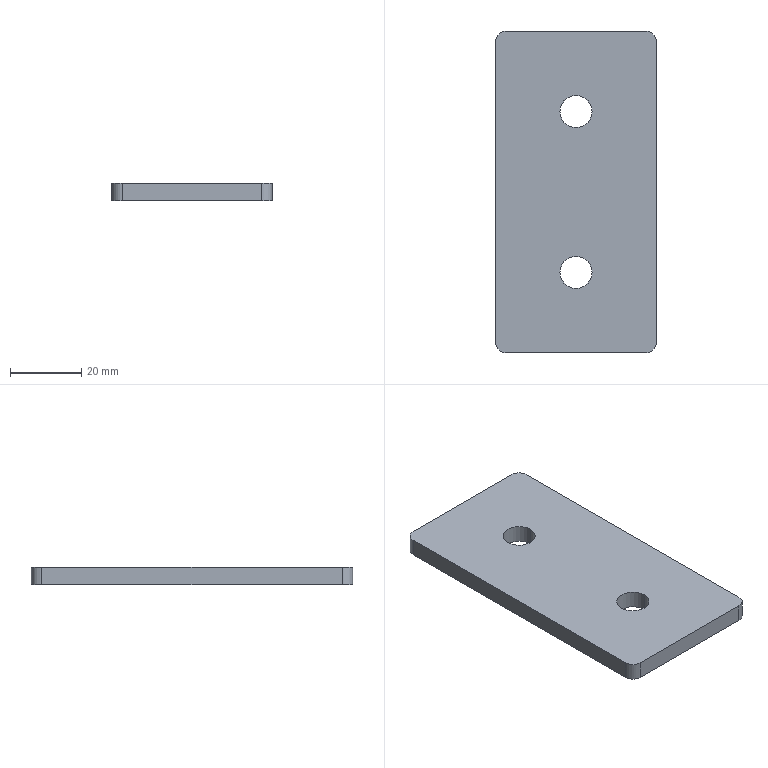Part | STEP file | 1 solid | 14 faces | box 45 x 90 x 5 mm | volume 19575 mm3 | cylinder 8 | plane 6 | commonest cylinder face diameters 6 x4 9 x4
STEP:
#1=CARTESIAN_POINT('',(0.,0.,0.));
#2=DIRECTION('',(0.,0.,1.));
#3=DIRECTION('',(1.,0.,0.));
#4=AXIS2_PLACEMENT_3D('',#1,#2,#3);
#5=CARTESIAN_POINT('',(-545.5,-331.5,5.));
#6=VERTEX_POINT('',#5);
#7=CARTESIAN_POINT('',(-554.5,-331.5,5.));
#8=VERTEX_POINT('',#7);
#9=CARTESIAN_POINT('',(-550.,-331.5,5.));
#10=DIRECTION('',(0.,0.,1.));
#11=DIRECTION('',(1.,0.,0.));
#12=AXIS2_PLACEMENT_3D('',#9,#10,#11);
#13=CIRCLE('',#12,4.5);
#14=CARTESIAN_POINT('',(-550.,-331.5,0.));
#15=DIRECTION('',(0.,0.,1.));
#16=DIRECTION('',(1.,0.,0.));
#17=AXIS2_PLACEMENT_3D('',#14,#15,#16);
#18=CYLINDRICAL_SURFACE('',#17,4.5);
#19=CARTESIAN_POINT('',(0.,5.));
#20=DIRECTION('',(1.,0.));
#21=VECTOR('',#20,1.);
#22=LINE('',#19,#21);
#23=(GEOMETRIC_REPRESENTATION_CONTEXT(2)PARAMETRIC_REPRESENTATION_CONTEXT()REPRESENTATION_CONTEXT('',''));
#24=DEFINITIONAL_REPRESENTATION('',(#22),#23);
#25=PCURVE('',#18,#24);
#26=CARTESIAN_POINT('',(-569.5,-267.,5.));
#27=DIRECTION('',(0.,0.,1.));
#28=DIRECTION('',(1.,0.,0.));
#29=AXIS2_PLACEMENT_3D('',#26,#27,#28);
#30=PLANE('',#29);
#31=CARTESIAN_POINT('',(19.5,-64.5));
#32=DIRECTION('',(1.,0.));
#33=AXIS2_PLACEMENT_2D('',#31,#32);
#34=CIRCLE('',#33,4.5);
#35=(GEOMETRIC_REPRESENTATION_CONTEXT(2)PARAMETRIC_REPRESENTATION_CONTEXT()REPRESENTATION_CONTEXT('',''));
#36=DEFINITIONAL_REPRESENTATION('',(#34),#35);
#37=PCURVE('',#30,#36);
#38=SURFACE_CURVE('',#13,(#25,#37),.PCURVE_S1.);
#39=EDGE_CURVE('',#6,#8,#38,.T.);
#40=ORIENTED_EDGE('',*,*,#39,.F.);
#41=CARTESIAN_POINT('',(-545.5,-331.5,0.));
#42=VERTEX_POINT('',#41);
#43=CARTESIAN_POINT('',(-545.5,-331.5,0.));
#44=DIRECTION('',(0.,0.,1.));
#45=VECTOR('',#44,1.);
#46=LINE('',#43,#45);
#47=CARTESIAN_POINT('',(0.,0.));
#48=DIRECTION('',(0.,1.));
#49=VECTOR('',#48,1.);
#50=LINE('',#47,#49);
#51=(GEOMETRIC_REPRESENTATION_CONTEXT(2)PARAMETRIC_REPRESENTATION_CONTEXT()REPRESENTATION_CONTEXT('',''));
#52=DEFINITIONAL_REPRESENTATION('',(#50),#51);
#53=PCURVE('',#18,#52);
#54=CARTESIAN_POINT('',(-550.,-331.5,0.));
#55=DIRECTION('',(0.,0.,1.));
#56=DIRECTION('',(1.,0.,0.));
#57=AXIS2_PLACEMENT_3D('',#54,#55,#56);
#58=CYLINDRICAL_SURFACE('',#57,4.5);
#59=CARTESIAN_POINT('',(6.283,0.));
#60=DIRECTION('',(0.,1.));
#61=VECTOR('',#60,1.);
#62=LINE('',#59,#61);
#63=(GEOMETRIC_REPRESENTATION_CONTEXT(2)PARAMETRIC_REPRESENTATION_CONTEXT()REPRESENTATION_CONTEXT('',''));
#64=DEFINITIONAL_REPRESENTATION('',(#62),#63);
#65=PCURVE('',#58,#64);
#66=SURFACE_CURVE('',#46,(#53,#65),.PCURVE_S1.);
#67=EDGE_CURVE('',#42,#6,#66,.T.);
#68=ORIENTED_EDGE('',*,*,#67,.F.);
#69=CARTESIAN_POINT('',(-554.5,-331.5,0.));
#70=VERTEX_POINT('',#69);
#71=CARTESIAN_POINT('',(-550.,-331.5,0.));
#72=DIRECTION('',(0.,0.,1.));
#73=DIRECTION('',(1.,0.,0.));
#74=AXIS2_PLACEMENT_3D('',#71,#72,#73);
#75=CIRCLE('',#74,4.5);
#76=CARTESIAN_POINT('',(0.,0.));
#77=DIRECTION('',(1.,0.));
#78=VECTOR('',#77,1.);
#79=LINE('',#76,#78);
#80=(GEOMETRIC_REPRESENTATION_CONTEXT(2)PARAMETRIC_REPRESENTATION_CONTEXT()REPRESENTATION_CONTEXT('',''));
#81=DEFINITIONAL_REPRESENTATION('',(#79),#80);
#82=PCURVE('',#18,#81);
#83=CARTESIAN_POINT('',(-569.5,-267.,0.));
#84=DIRECTION('',(0.,0.,1.));
#85=DIRECTION('',(1.,0.,0.));
#86=AXIS2_PLACEMENT_3D('',#83,#84,#85);
#87=PLANE('',#86);
#88=CARTESIAN_POINT('',(19.5,-64.5));
#89=DIRECTION('',(1.,0.));
#90=AXIS2_PLACEMENT_2D('',#88,#89);
#91=CIRCLE('',#90,4.5);
#92=(GEOMETRIC_REPRESENTATION_CONTEXT(2)PARAMETRIC_REPRESENTATION_CONTEXT()REPRESENTATION_CONTEXT('',''));
#93=DEFINITIONAL_REPRESENTATION('',(#91),#92);
#94=PCURVE('',#87,#93);
#95=SURFACE_CURVE('',#75,(#82,#94),.PCURVE_S1.);
#96=EDGE_CURVE('',#42,#70,#95,.T.);
#97=ORIENTED_EDGE('',*,*,#96,.T.);
#98=CARTESIAN_POINT('',(-554.5,-331.5,0.));
#99=DIRECTION('',(0.,0.,1.));
#100=VECTOR('',#99,1.);
#101=LINE('',#98,#100);
#102=CARTESIAN_POINT('',(3.142,0.));
#103=DIRECTION('',(0.,1.));
#104=VECTOR('',#103,1.);
#105=LINE('',#102,#104);
#106=(GEOMETRIC_REPRESENTATION_CONTEXT(2)PARAMETRIC_REPRESENTATION_CONTEXT()REPRESENTATION_CONTEXT('',''));
#107=DEFINITIONAL_REPRESENTATION('',(#105),#106);
#108=PCURVE('',#18,#107);
#109=CARTESIAN_POINT('',(3.142,0.));
#110=DIRECTION('',(0.,1.));
#111=VECTOR('',#110,1.);
#112=LINE('',#109,#111);
#113=(GEOMETRIC_REPRESENTATION_CONTEXT(2)PARAMETRIC_REPRESENTATION_CONTEXT()REPRESENTATION_CONTEXT('',''));
#114=DEFINITIONAL_REPRESENTATION('',(#112),#113);
#115=PCURVE('',#58,#114);
#116=SURFACE_CURVE('',#101,(#108,#115),.PCURVE_S1.);
#117=EDGE_CURVE('',#70,#8,#116,.T.);
#118=ORIENTED_EDGE('',*,*,#117,.T.);
#119=EDGE_LOOP('',(#40,#68,#97,#118));
#120=FACE_BOUND('',#119,.F.);
#121=ADVANCED_FACE('',(#120),#18,.F.);
#122=CARTESIAN_POINT('',(-545.5,-286.5,5.));
#123=VERTEX_POINT('',#122);
#124=CARTESIAN_POINT('',(-554.5,-286.5,5.));
#125=VERTEX_POINT('',#124);
#126=CARTESIAN_POINT('',(-550.,-286.5,5.));
#127=DIRECTION('',(0.,0.,1.));
#128=DIRECTION('',(1.,0.,0.));
#129=AXIS2_PLACEMENT_3D('',#126,#127,#128);
#130=CIRCLE('',#129,4.5);
#131=CARTESIAN_POINT('',(-550.,-286.5,0.));
#132=DIRECTION('',(0.,0.,1.));
#133=DIRECTION('',(1.,0.,0.));
#134=AXIS2_PLACEMENT_3D('',#131,#132,#133);
#135=CYLINDRICAL_SURFACE('',#134,4.5);
#136=CARTESIAN_POINT('',(0.,5.));
#137=DIRECTION('',(1.,0.));
#138=VECTOR('',#137,1.);
#139=LINE('',#136,#138);
#140=(GEOMETRIC_REPRESENTATION_CONTEXT(2)PARAMETRIC_REPRESENTATION_CONTEXT()REPRESENTATION_CONTEXT('',''));
#141=DEFINITIONAL_REPRESENTATION('',(#139),#140);
#142=PCURVE('',#135,#141);
#143=CARTESIAN_POINT('',(19.5,-19.5));
#144=DIRECTION('',(1.,0.));
#145=AXIS2_PLACEMENT_2D('',#143,#144);
#146=CIRCLE('',#145,4.5);
#147=(GEOMETRIC_REPRESENTATION_CONTEXT(2)PARAMETRIC_REPRESENTATION_CONTEXT()REPRESENTATION_CONTEXT('',''));
#148=DEFINITIONAL_REPRESENTATION('',(#146),#147);
#149=PCURVE('',#30,#148);
#150=SURFACE_CURVE('',#130,(#142,#149),.PCURVE_S1.);
#151=EDGE_CURVE('',#123,#125,#150,.T.);
#152=ORIENTED_EDGE('',*,*,#151,.F.);
#153=CARTESIAN_POINT('',(-545.5,-286.5,0.));
#154=VERTEX_POINT('',#153);
#155=CARTESIAN_POINT('',(-545.5,-286.5,0.));
#156=DIRECTION('',(0.,0.,1.));
#157=VECTOR('',#156,1.);
#158=LINE('',#155,#157);
#159=CARTESIAN_POINT('',(0.,0.));
#160=DIRECTION('',(0.,1.));
#161=VECTOR('',#160,1.);
#162=LINE('',#159,#161);
#163=(GEOMETRIC_REPRESENTATION_CONTEXT(2)PARAMETRIC_REPRESENTATION_CONTEXT()REPRESENTATION_CONTEXT('',''));
#164=DEFINITIONAL_REPRESENTATION('',(#162),#163);
#165=PCURVE('',#135,#164);
#166=CARTESIAN_POINT('',(-550.,-286.5,0.));
#167=DIRECTION('',(0.,0.,1.));
#168=DIRECTION('',(1.,0.,0.));
#169=AXIS2_PLACEMENT_3D('',#166,#167,#168);
#170=CYLINDRICAL_SURFACE('',#169,4.5);
#171=CARTESIAN_POINT('',(6.283,0.));
#172=DIRECTION('',(0.,1.));
#173=VECTOR('',#172,1.);
#174=LINE('',#171,#173);
#175=(GEOMETRIC_REPRESENTATION_CONTEXT(2)PARAMETRIC_REPRESENTATION_CONTEXT()REPRESENTATION_CONTEXT('',''));
#176=DEFINITIONAL_REPRESENTATION('',(#174),#175);
#177=PCURVE('',#170,#176);
#178=SURFACE_CURVE('',#158,(#165,#177),.PCURVE_S1.);
#179=EDGE_CURVE('',#154,#123,#178,.T.);
#180=ORIENTED_EDGE('',*,*,#179,.F.);
#181=CARTESIAN_POINT('',(-554.5,-286.5,0.));
#182=VERTEX_POINT('',#181);
#183=CARTESIAN_POINT('',(-550.,-286.5,0.));
#184=DIRECTION('',(0.,0.,1.));
#185=DIRECTION('',(1.,0.,0.));
#186=AXIS2_PLACEMENT_3D('',#183,#184,#185);
#187=CIRCLE('',#186,4.5);
#188=CARTESIAN_POINT('',(0.,0.));
#189=DIRECTION('',(1.,0.));
#190=VECTOR('',#189,1.);
#191=LINE('',#188,#190);
#192=(GEOMETRIC_REPRESENTATION_CONTEXT(2)PARAMETRIC_REPRESENTATION_CONTEXT()REPRESENTATION_CONTEXT('',''));
#193=DEFINITIONAL_REPRESENTATION('',(#191),#192);
#194=PCURVE('',#135,#193);
#195=CARTESIAN_POINT('',(19.5,-19.5));
#196=DIRECTION('',(1.,0.));
#197=AXIS2_PLACEMENT_2D('',#195,#196);
#198=CIRCLE('',#197,4.5);
#199=(GEOMETRIC_REPRESENTATION_CONTEXT(2)PARAMETRIC_REPRESENTATION_CONTEXT()REPRESENTATION_CONTEXT('',''));
#200=DEFINITIONAL_REPRESENTATION('',(#198),#199);
#201=PCURVE('',#87,#200);
#202=SURFACE_CURVE('',#187,(#194,#201),.PCURVE_S1.);
#203=EDGE_CURVE('',#154,#182,#202,.T.);
#204=ORIENTED_EDGE('',*,*,#203,.T.);
#205=CARTESIAN_POINT('',(-554.5,-286.5,0.));
#206=DIRECTION('',(0.,0.,1.));
#207=VECTOR('',#206,1.);
#208=LINE('',#205,#207);
#209=CARTESIAN_POINT('',(3.142,0.));
#210=DIRECTION('',(0.,1.));
#211=VECTOR('',#210,1.);
#212=LINE('',#209,#211);
#213=(GEOMETRIC_REPRESENTATION_CONTEXT(2)PARAMETRIC_REPRESENTATION_CONTEXT()REPRESENTATION_CONTEXT('',''));
#214=DEFINITIONAL_REPRESENTATION('',(#212),#213);
#215=PCURVE('',#135,#214);
#216=CARTESIAN_POINT('',(3.142,0.));
#217=DIRECTION('',(0.,1.));
#218=VECTOR('',#217,1.);
#219=LINE('',#216,#218);
#220=(GEOMETRIC_REPRESENTATION_CONTEXT(2)PARAMETRIC_REPRESENTATION_CONTEXT()REPRESENTATION_CONTEXT('',''));
#221=DEFINITIONAL_REPRESENTATION('',(#219),#220);
#222=PCURVE('',#170,#221);
#223=SURFACE_CURVE('',#208,(#215,#222),.PCURVE_S1.);
#224=EDGE_CURVE('',#182,#125,#223,.T.);
#225=ORIENTED_EDGE('',*,*,#224,.T.);
#226=EDGE_LOOP('',(#152,#180,#204,#225));
#227=FACE_BOUND('',#226,.F.);
#228=ADVANCED_FACE('',(#227),#135,.F.);
#229=ORIENTED_EDGE('',*,*,#203,.T.);
#230=CARTESIAN_POINT('',(-550.,-286.5,0.));
#231=DIRECTION('',(0.,0.,1.));
#232=DIRECTION('',(1.,0.,0.));
#233=AXIS2_PLACEMENT_3D('',#230,#231,#232);
#234=CIRCLE('',#233,4.5);
#235=CARTESIAN_POINT('',(19.5,-19.5));
#236=DIRECTION('',(1.,0.));
#237=AXIS2_PLACEMENT_2D('',#235,#236);
#238=CIRCLE('',#237,4.5);
#239=(GEOMETRIC_REPRESENTATION_CONTEXT(2)PARAMETRIC_REPRESENTATION_CONTEXT()REPRESENTATION_CONTEXT('',''));
#240=DEFINITIONAL_REPRESENTATION('',(#238),#239);
#241=PCURVE('',#87,#240);
#242=CARTESIAN_POINT('',(0.,0.));
#243=DIRECTION('',(1.,0.));
#244=VECTOR('',#243,1.);
#245=LINE('',#242,#244);
#246=(GEOMETRIC_REPRESENTATION_CONTEXT(2)PARAMETRIC_REPRESENTATION_CONTEXT()REPRESENTATION_CONTEXT('',''));
#247=DEFINITIONAL_REPRESENTATION('',(#245),#246);
#248=PCURVE('',#170,#247);
#249=SURFACE_CURVE('',#234,(#241,#248),.PCURVE_S1.);
#250=EDGE_CURVE('',#182,#154,#249,.T.);
#251=ORIENTED_EDGE('',*,*,#250,.T.);
#252=EDGE_LOOP('',(#229,#251));
#253=FACE_BOUND('',#252,.T.);
#254=ORIENTED_EDGE('',*,*,#96,.T.);
#255=CARTESIAN_POINT('',(-550.,-331.5,0.));
#256=DIRECTION('',(0.,0.,1.));
#257=DIRECTION('',(1.,0.,0.));
#258=AXIS2_PLACEMENT_3D('',#255,#256,#257);
#259=CIRCLE('',#258,4.5);
#260=CARTESIAN_POINT('',(19.5,-64.5));
#261=DIRECTION('',(1.,0.));
#262=AXIS2_PLACEMENT_2D('',#260,#261);
#263=CIRCLE('',#262,4.5);
#264=(GEOMETRIC_REPRESENTATION_CONTEXT(2)PARAMETRIC_REPRESENTATION_CONTEXT()REPRESENTATION_CONTEXT('',''));
#265=DEFINITIONAL_REPRESENTATION('',(#263),#264);
#266=PCURVE('',#87,#265);
#267=CARTESIAN_POINT('',(0.,0.));
#268=DIRECTION('',(1.,0.));
#269=VECTOR('',#268,1.);
#270=LINE('',#267,#269);
#271=(GEOMETRIC_REPRESENTATION_CONTEXT(2)PARAMETRIC_REPRESENTATION_CONTEXT()REPRESENTATION_CONTEXT('',''));
#272=DEFINITIONAL_REPRESENTATION('',(#270),#271);
#273=PCURVE('',#58,#272);
#274=SURFACE_CURVE('',#259,(#266,#273),.PCURVE_S1.);
#275=EDGE_CURVE('',#70,#42,#274,.T.);
#276=ORIENTED_EDGE('',*,*,#275,.T.);
#277=EDGE_LOOP('',(#254,#276));
#278=FACE_BOUND('',#277,.T.);
#279=CARTESIAN_POINT('',(-569.5,-264.,0.));
#280=VERTEX_POINT('',#279);
#281=CARTESIAN_POINT('',(-572.5,-267.,0.));
#282=VERTEX_POINT('',#281);
#283=CARTESIAN_POINT('',(-569.5,-267.,0.));
#284=DIRECTION('',(0.,0.,1.));
#285=DIRECTION('',(1.,0.,0.));
#286=AXIS2_PLACEMENT_3D('',#283,#284,#285);
#287=CIRCLE('',#286,3.);
#288=CARTESIAN_POINT('',(0.,0.));
#289=DIRECTION('',(1.,0.));
#290=AXIS2_PLACEMENT_2D('',#288,#289);
#291=CIRCLE('',#290,3.);
#292=(GEOMETRIC_REPRESENTATION_CONTEXT(2)PARAMETRIC_REPRESENTATION_CONTEXT()REPRESENTATION_CONTEXT('',''));
#293=DEFINITIONAL_REPRESENTATION('',(#291),#292);
#294=PCURVE('',#87,#293);
#295=CARTESIAN_POINT('',(-569.5,-267.,5.));
#296=DIRECTION('',(0.,0.,-1.));
#297=DIRECTION('',(-1.,0.,0.));
#298=AXIS2_PLACEMENT_3D('',#295,#296,#297);
#299=CYLINDRICAL_SURFACE('',#298,3.);
#300=CARTESIAN_POINT('',(3.142,5.));
#301=DIRECTION('',(-1.,0.));
#302=VECTOR('',#301,1.);
#303=LINE('',#300,#302);
#304=(GEOMETRIC_REPRESENTATION_CONTEXT(2)PARAMETRIC_REPRESENTATION_CONTEXT()REPRESENTATION_CONTEXT('',''));
#305=DEFINITIONAL_REPRESENTATION('',(#303),#304);
#306=PCURVE('',#299,#305);
#307=SURFACE_CURVE('',#287,(#294,#306),.PCURVE_S1.);
#308=EDGE_CURVE('',#280,#282,#307,.T.);
#309=ORIENTED_EDGE('',*,*,#308,.F.);
#310=CARTESIAN_POINT('',(-530.5,-264.,0.));
#311=VERTEX_POINT('',#310);
#312=CARTESIAN_POINT('',(-530.5,-264.,0.));
#313=DIRECTION('',(-1.,0.,0.));
#314=VECTOR('',#313,1.);
#315=LINE('',#312,#314);
#316=CARTESIAN_POINT('',(39.,3.));
#317=DIRECTION('',(-1.,0.));
#318=VECTOR('',#317,1.);
#319=LINE('',#316,#318);
#320=(GEOMETRIC_REPRESENTATION_CONTEXT(2)PARAMETRIC_REPRESENTATION_CONTEXT()REPRESENTATION_CONTEXT('',''));
#321=DEFINITIONAL_REPRESENTATION('',(#319),#320);
#322=PCURVE('',#87,#321);
#323=CARTESIAN_POINT('',(-530.5,-264.,5.));
#324=DIRECTION('',(0.,-1.,0.));
#325=DIRECTION('',(0.,0.,-1.));
#326=AXIS2_PLACEMENT_3D('',#323,#324,#325);
#327=PLANE('',#326);
#328=CARTESIAN_POINT('',(5.,0.));
#329=DIRECTION('',(0.,-1.));
#330=VECTOR('',#329,1.);
#331=LINE('',#328,#330);
#332=(GEOMETRIC_REPRESENTATION_CONTEXT(2)PARAMETRIC_REPRESENTATION_CONTEXT()REPRESENTATION_CONTEXT('',''));
#333=DEFINITIONAL_REPRESENTATION('',(#331),#332);
#334=PCURVE('',#327,#333);
#335=SURFACE_CURVE('',#315,(#322,#334),.PCURVE_S1.);
#336=EDGE_CURVE('',#311,#280,#335,.T.);
#337=ORIENTED_EDGE('',*,*,#336,.F.);
#338=CARTESIAN_POINT('',(-527.5,-267.,0.));
#339=VERTEX_POINT('',#338);
#340=CARTESIAN_POINT('',(-530.5,-267.,0.));
#341=DIRECTION('',(0.,0.,1.));
#342=DIRECTION('',(-1.,0.,0.));
#343=AXIS2_PLACEMENT_3D('',#340,#341,#342);
#344=CIRCLE('',#343,3.);
#345=CARTESIAN_POINT('',(39.,0.));
#346=DIRECTION('',(-1.,0.));
#347=AXIS2_PLACEMENT_2D('',#345,#346);
#348=CIRCLE('',#347,3.);
#349=(GEOMETRIC_REPRESENTATION_CONTEXT(2)PARAMETRIC_REPRESENTATION_CONTEXT()REPRESENTATION_CONTEXT('',''));
#350=DEFINITIONAL_REPRESENTATION('',(#348),#349);
#351=PCURVE('',#87,#350);
#352=CARTESIAN_POINT('',(-530.5,-267.,5.));
#353=DIRECTION('',(0.,0.,-1.));
#354=DIRECTION('',(-1.,0.,0.));
#355=AXIS2_PLACEMENT_3D('',#352,#353,#354);
#356=CYLINDRICAL_SURFACE('',#355,3.);
#357=CARTESIAN_POINT('',(6.283,5.));
#358=DIRECTION('',(-1.,0.));
#359=VECTOR('',#358,1.);
#360=LINE('',#357,#359);
#361=(GEOMETRIC_REPRESENTATION_CONTEXT(2)PARAMETRIC_REPRESENTATION_CONTEXT()REPRESENTATION_CONTEXT('',''));
#362=DEFINITIONAL_REPRESENTATION('',(#360),#361);
#363=PCURVE('',#356,#362);
#364=SURFACE_CURVE('',#344,(#351,#363),.PCURVE_S1.);
#365=EDGE_CURVE('',#339,#311,#364,.T.);
#366=ORIENTED_EDGE('',*,*,#365,.F.);
#367=CARTESIAN_POINT('',(-527.5,-351.,0.));
#368=VERTEX_POINT('',#367);
#369=CARTESIAN_POINT('',(-527.5,-267.,0.));
#370=DIRECTION('',(0.,1.,0.));
#371=VECTOR('',#370,1.);
#372=LINE('',#369,#371);
#373=CARTESIAN_POINT('',(42.,0.));
#374=DIRECTION('',(0.,1.));
#375=VECTOR('',#374,1.);
#376=LINE('',#373,#375);
#377=(GEOMETRIC_REPRESENTATION_CONTEXT(2)PARAMETRIC_REPRESENTATION_CONTEXT()REPRESENTATION_CONTEXT('',''));
#378=DEFINITIONAL_REPRESENTATION('',(#376),#377);
#379=PCURVE('',#87,#378);
#380=CARTESIAN_POINT('',(-527.5,-267.,5.));
#381=DIRECTION('',(-1.,0.,0.));
#382=DIRECTION('',(0.,0.,1.));
#383=AXIS2_PLACEMENT_3D('',#380,#381,#382);
#384=PLANE('',#383);
#385=CARTESIAN_POINT('',(-5.,0.));
#386=DIRECTION('',(0.,1.));
#387=VECTOR('',#386,1.);
#388=LINE('',#385,#387);
#389=(GEOMETRIC_REPRESENTATION_CONTEXT(2)PARAMETRIC_REPRESENTATION_CONTEXT()REPRESENTATION_CONTEXT('',''));
#390=DEFINITIONAL_REPRESENTATION('',(#388),#389);
#391=PCURVE('',#384,#390);
#392=SURFACE_CURVE('',#372,(#379,#391),.PCURVE_S1.);
#393=EDGE_CURVE('',#368,#339,#392,.T.);
#394=ORIENTED_EDGE('',*,*,#393,.F.);
#395=CARTESIAN_POINT('',(-530.5,-354.,0.));
#396=VERTEX_POINT('',#395);
#397=CARTESIAN_POINT('',(-530.5,-351.,0.));
#398=DIRECTION('',(0.,0.,1.));
#399=DIRECTION('',(-1.,0.,0.));
#400=AXIS2_PLACEMENT_3D('',#397,#398,#399);
#401=CIRCLE('',#400,3.);
#402=CARTESIAN_POINT('',(39.,-84.));
#403=DIRECTION('',(-1.,0.));
#404=AXIS2_PLACEMENT_2D('',#402,#403);
#405=CIRCLE('',#404,3.);
#406=(GEOMETRIC_REPRESENTATION_CONTEXT(2)PARAMETRIC_REPRESENTATION_CONTEXT()REPRESENTATION_CONTEXT('',''));
#407=DEFINITIONAL_REPRESENTATION('',(#405),#406);
#408=PCURVE('',#87,#407);
#409=CARTESIAN_POINT('',(-530.5,-351.,5.));
#410=DIRECTION('',(0.,0.,-1.));
#411=DIRECTION('',(-1.,0.,0.));
#412=AXIS2_PLACEMENT_3D('',#409,#410,#411);
#413=CYLINDRICAL_SURFACE('',#412,3.);
#414=CARTESIAN_POINT('',(6.283,5.));
#415=DIRECTION('',(-1.,0.));
#416=VECTOR('',#415,1.);
#417=LINE('',#414,#416);
#418=(GEOMETRIC_REPRESENTATION_CONTEXT(2)PARAMETRIC_REPRESENTATION_CONTEXT()REPRESENTATION_CONTEXT('',''));
#419=DEFINITIONAL_REPRESENTATION('',(#417),#418);
#420=PCURVE('',#413,#419);
#421=SURFACE_CURVE('',#401,(#408,#420),.PCURVE_S1.);
#422=EDGE_CURVE('',#396,#368,#421,.T.);
#423=ORIENTED_EDGE('',*,*,#422,.F.);
#424=CARTESIAN_POINT('',(-569.5,-354.,0.));
#425=VERTEX_POINT('',#424);
#426=CARTESIAN_POINT('',(-530.5,-354.,0.));
#427=DIRECTION('',(1.,0.,0.));
#428=VECTOR('',#427,1.);
#429=LINE('',#426,#428);
#430=CARTESIAN_POINT('',(39.,-87.));
#431=DIRECTION('',(1.,0.));
#432=VECTOR('',#431,1.);
#433=LINE('',#430,#432);
#434=(GEOMETRIC_REPRESENTATION_CONTEXT(2)PARAMETRIC_REPRESENTATION_CONTEXT()REPRESENTATION_CONTEXT('',''));
#435=DEFINITIONAL_REPRESENTATION('',(#433),#434);
#436=PCURVE('',#87,#435);
#437=CARTESIAN_POINT('',(-530.5,-354.,5.));
#438=DIRECTION('',(0.,1.,0.));
#439=DIRECTION('',(1.,0.,0.));
#440=AXIS2_PLACEMENT_3D('',#437,#438,#439);
#441=PLANE('',#440);
#442=CARTESIAN_POINT('',(0.,5.));
#443=DIRECTION('',(1.,0.));
#444=VECTOR('',#443,1.);
#445=LINE('',#442,#444);
#446=(GEOMETRIC_REPRESENTATION_CONTEXT(2)PARAMETRIC_REPRESENTATION_CONTEXT()REPRESENTATION_CONTEXT('',''));
#447=DEFINITIONAL_REPRESENTATION('',(#445),#446);
#448=PCURVE('',#441,#447);
#449=SURFACE_CURVE('',#429,(#436,#448),.PCURVE_S1.);
#450=EDGE_CURVE('',#425,#396,#449,.T.);
#451=ORIENTED_EDGE('',*,*,#450,.F.);
#452=CARTESIAN_POINT('',(-572.5,-351.,0.));
#453=VERTEX_POINT('',#452);
#454=CARTESIAN_POINT('',(-569.5,-351.,0.));
#455=DIRECTION('',(0.,0.,1.));
#456=DIRECTION('',(-1.,0.,0.));
#457=AXIS2_PLACEMENT_3D('',#454,#455,#456);
#458=CIRCLE('',#457,3.);
#459=CARTESIAN_POINT('',(0.,-84.));
#460=DIRECTION('',(-1.,0.));
#461=AXIS2_PLACEMENT_2D('',#459,#460);
#462=CIRCLE('',#461,3.);
#463=(GEOMETRIC_REPRESENTATION_CONTEXT(2)PARAMETRIC_REPRESENTATION_CONTEXT()REPRESENTATION_CONTEXT('',''));
#464=DEFINITIONAL_REPRESENTATION('',(#462),#463);
#465=PCURVE('',#87,#464);
#466=CARTESIAN_POINT('',(-569.5,-351.,5.));
#467=DIRECTION('',(0.,0.,-1.));
#468=DIRECTION('',(-1.,0.,0.));
#469=AXIS2_PLACEMENT_3D('',#466,#467,#468);
#470=CYLINDRICAL_SURFACE('',#469,3.);
#471=CARTESIAN_POINT('',(6.283,5.));
#472=DIRECTION('',(-1.,0.));
#473=VECTOR('',#472,1.);
#474=LINE('',#471,#473);
#475=(GEOMETRIC_REPRESENTATION_CONTEXT(2)PARAMETRIC_REPRESENTATION_CONTEXT()REPRESENTATION_CONTEXT('',''));
#476=DEFINITIONAL_REPRESENTATION('',(#474),#475);
#477=PCURVE('',#470,#476);
#478=SURFACE_CURVE('',#458,(#465,#477),.PCURVE_S1.);
#479=EDGE_CURVE('',#453,#425,#478,.T.);
#480=ORIENTED_EDGE('',*,*,#479,.F.);
#481=CARTESIAN_POINT('',(-572.5,-267.,0.));
#482=DIRECTION('',(0.,-1.,0.));
#483=VECTOR('',#482,1.);
#484=LINE('',#481,#483);
#485=CARTESIAN_POINT('',(-3.,0.));
#486=DIRECTION('',(0.,-1.));
#487=VECTOR('',#486,1.);
#488=LINE('',#485,#487);
#489=(GEOMETRIC_REPRESENTATION_CONTEXT(2)PARAMETRIC_REPRESENTATION_CONTEXT()REPRESENTATION_CONTEXT('',''));
#490=DEFINITIONAL_REPRESENTATION('',(#488),#489);
#491=PCURVE('',#87,#490);
#492=CARTESIAN_POINT('',(-572.5,-267.,5.));
#493=DIRECTION('',(1.,0.,0.));
#494=DIRECTION('',(0.,1.,0.));
#495=AXIS2_PLACEMENT_3D('',#492,#493,#494);
#496=PLANE('',#495);
#497=CARTESIAN_POINT('',(0.,-5.));
#498=DIRECTION('',(-1.,0.));
#499=VECTOR('',#498,1.);
#500=LINE('',#497,#499);
#501=(GEOMETRIC_REPRESENTATION_CONTEXT(2)PARAMETRIC_REPRESENTATION_CONTEXT()REPRESENTATION_CONTEXT('',''));
#502=DEFINITIONAL_REPRESENTATION('',(#500),#501);
#503=PCURVE('',#496,#502);
#504=SURFACE_CURVE('',#484,(#491,#503),.PCURVE_S1.);
#505=EDGE_CURVE('',#282,#453,#504,.T.);
#506=ORIENTED_EDGE('',*,*,#505,.F.);
#507=EDGE_LOOP('',(#309,#337,#366,#394,#423,#451,#480,#506));
#508=FACE_BOUND('',#507,.T.);
#509=ADVANCED_FACE('',(#253,#278,#508),#87,.F.);
#510=ORIENTED_EDGE('',*,*,#151,.F.);
#511=CARTESIAN_POINT('',(-550.,-286.5,5.));
#512=DIRECTION('',(0.,0.,1.));
#513=DIRECTION('',(1.,0.,0.));
#514=AXIS2_PLACEMENT_3D('',#511,#512,#513);
#515=CIRCLE('',#514,4.5);
#516=CARTESIAN_POINT('',(19.5,-19.5));
#517=DIRECTION('',(1.,0.));
#518=AXIS2_PLACEMENT_2D('',#516,#517);
#519=CIRCLE('',#518,4.5);
#520=(GEOMETRIC_REPRESENTATION_CONTEXT(2)PARAMETRIC_REPRESENTATION_CONTEXT()REPRESENTATION_CONTEXT('',''));
#521=DEFINITIONAL_REPRESENTATION('',(#519),#520);
#522=PCURVE('',#30,#521);
#523=CARTESIAN_POINT('',(0.,5.));
#524=DIRECTION('',(1.,0.));
#525=VECTOR('',#524,1.);
#526=LINE('',#523,#525);
#527=(GEOMETRIC_REPRESENTATION_CONTEXT(2)PARAMETRIC_REPRESENTATION_CONTEXT()REPRESENTATION_CONTEXT('',''));
#528=DEFINITIONAL_REPRESENTATION('',(#526),#527);
#529=PCURVE('',#170,#528);
#530=SURFACE_CURVE('',#515,(#522,#529),.PCURVE_S1.);
#531=EDGE_CURVE('',#125,#123,#530,.T.);
#532=ORIENTED_EDGE('',*,*,#531,.F.);
#533=EDGE_LOOP('',(#510,#532));
#534=FACE_BOUND('',#533,.T.);
#535=ORIENTED_EDGE('',*,*,#39,.F.);
#536=CARTESIAN_POINT('',(-550.,-331.5,5.));
#537=DIRECTION('',(0.,0.,1.));
#538=DIRECTION('',(1.,0.,0.));
#539=AXIS2_PLACEMENT_3D('',#536,#537,#538);
#540=CIRCLE('',#539,4.5);
#541=CARTESIAN_POINT('',(19.5,-64.5));
#542=DIRECTION('',(1.,0.));
#543=AXIS2_PLACEMENT_2D('',#541,#542);
#544=CIRCLE('',#543,4.5);
#545=(GEOMETRIC_REPRESENTATION_CONTEXT(2)PARAMETRIC_REPRESENTATION_CONTEXT()REPRESENTATION_CONTEXT('',''));
#546=DEFINITIONAL_REPRESENTATION('',(#544),#545);
#547=PCURVE('',#30,#546);
#548=CARTESIAN_POINT('',(0.,5.));
#549=DIRECTION('',(1.,0.));
#550=VECTOR('',#549,1.);
#551=LINE('',#548,#550);
#552=(GEOMETRIC_REPRESENTATION_CONTEXT(2)PARAMETRIC_REPRESENTATION_CONTEXT()REPRESENTATION_CONTEXT('',''));
#553=DEFINITIONAL_REPRESENTATION('',(#551),#552);
#554=PCURVE('',#58,#553);
#555=SURFACE_CURVE('',#540,(#547,#554),.PCURVE_S1.);
#556=EDGE_CURVE('',#8,#6,#555,.T.);
#557=ORIENTED_EDGE('',*,*,#556,.F.);
#558=EDGE_LOOP('',(#535,#557));
#559=FACE_BOUND('',#558,.T.);
#560=CARTESIAN_POINT('',(-569.5,-264.,5.));
#561=VERTEX_POINT('',#560);
#562=CARTESIAN_POINT('',(-572.5,-267.,5.));
#563=VERTEX_POINT('',#562);
#564=CARTESIAN_POINT('',(-569.5,-267.,5.));
#565=DIRECTION('',(0.,0.,1.));
#566=DIRECTION('',(1.,0.,0.));
#567=AXIS2_PLACEMENT_3D('',#564,#565,#566);
#568=CIRCLE('',#567,3.);
#569=CARTESIAN_POINT('',(0.,0.));
#570=DIRECTION('',(1.,0.));
#571=AXIS2_PLACEMENT_2D('',#569,#570);
#572=CIRCLE('',#571,3.);
#573=(GEOMETRIC_REPRESENTATION_CONTEXT(2)PARAMETRIC_REPRESENTATION_CONTEXT()REPRESENTATION_CONTEXT('',''));
#574=DEFINITIONAL_REPRESENTATION('',(#572),#573);
#575=PCURVE('',#30,#574);
#576=CARTESIAN_POINT('',(3.142,0.));
#577=DIRECTION('',(-1.,0.));
#578=VECTOR('',#577,1.);
#579=LINE('',#576,#578);
#580=(GEOMETRIC_REPRESENTATION_CONTEXT(2)PARAMETRIC_REPRESENTATION_CONTEXT()REPRESENTATION_CONTEXT('',''));
#581=DEFINITIONAL_REPRESENTATION('',(#579),#580);
#582=PCURVE('',#299,#581);
#583=SURFACE_CURVE('',#568,(#575,#582),.PCURVE_S1.);
#584=EDGE_CURVE('',#561,#563,#583,.T.);
#585=ORIENTED_EDGE('',*,*,#584,.T.);
#586=CARTESIAN_POINT('',(-572.5,-351.,5.));
#587=VERTEX_POINT('',#586);
#588=CARTESIAN_POINT('',(-572.5,-267.,5.));
#589=DIRECTION('',(0.,-1.,0.));
#590=VECTOR('',#589,1.);
#591=LINE('',#588,#590);
#592=CARTESIAN_POINT('',(-3.,0.));
#593=DIRECTION('',(0.,-1.));
#594=VECTOR('',#593,1.);
#595=LINE('',#592,#594);
#596=(GEOMETRIC_REPRESENTATION_CONTEXT(2)PARAMETRIC_REPRESENTATION_CONTEXT()REPRESENTATION_CONTEXT('',''));
#597=DEFINITIONAL_REPRESENTATION('',(#595),#596);
#598=PCURVE('',#30,#597);
#599=CARTESIAN_POINT('',(0.,0.));
#600=DIRECTION('',(-1.,0.));
#601=VECTOR('',#600,1.);
#602=LINE('',#599,#601);
#603=(GEOMETRIC_REPRESENTATION_CONTEXT(2)PARAMETRIC_REPRESENTATION_CONTEXT()REPRESENTATION_CONTEXT('',''));
#604=DEFINITIONAL_REPRESENTATION('',(#602),#603);
#605=PCURVE('',#496,#604);
#606=SURFACE_CURVE('',#591,(#598,#605),.PCURVE_S1.);
#607=EDGE_CURVE('',#563,#587,#606,.T.);
#608=ORIENTED_EDGE('',*,*,#607,.T.);
#609=CARTESIAN_POINT('',(-569.5,-354.,5.));
#610=VERTEX_POINT('',#609);
#611=CARTESIAN_POINT('',(-569.5,-351.,5.));
#612=DIRECTION('',(0.,0.,1.));
#613=DIRECTION('',(-1.,0.,0.));
#614=AXIS2_PLACEMENT_3D('',#611,#612,#613);
#615=CIRCLE('',#614,3.);
#616=CARTESIAN_POINT('',(0.,-84.));
#617=DIRECTION('',(-1.,0.));
#618=AXIS2_PLACEMENT_2D('',#616,#617);
#619=CIRCLE('',#618,3.);
#620=(GEOMETRIC_REPRESENTATION_CONTEXT(2)PARAMETRIC_REPRESENTATION_CONTEXT()REPRESENTATION_CONTEXT('',''));
#621=DEFINITIONAL_REPRESENTATION('',(#619),#620);
#622=PCURVE('',#30,#621);
#623=CARTESIAN_POINT('',(6.283,0.));
#624=DIRECTION('',(-1.,0.));
#625=VECTOR('',#624,1.);
#626=LINE('',#623,#625);
#627=(GEOMETRIC_REPRESENTATION_CONTEXT(2)PARAMETRIC_REPRESENTATION_CONTEXT()REPRESENTATION_CONTEXT('',''));
#628=DEFINITIONAL_REPRESENTATION('',(#626),#627);
#629=PCURVE('',#470,#628);
#630=SURFACE_CURVE('',#615,(#622,#629),.PCURVE_S1.);
#631=EDGE_CURVE('',#587,#610,#630,.T.);
#632=ORIENTED_EDGE('',*,*,#631,.T.);
#633=CARTESIAN_POINT('',(-530.5,-354.,5.));
#634=VERTEX_POINT('',#633);
#635=CARTESIAN_POINT('',(-530.5,-354.,5.));
#636=DIRECTION('',(1.,0.,0.));
#637=VECTOR('',#636,1.);
#638=LINE('',#635,#637);
#639=CARTESIAN_POINT('',(39.,-87.));
#640=DIRECTION('',(1.,0.));
#641=VECTOR('',#640,1.);
#642=LINE('',#639,#641);
#643=(GEOMETRIC_REPRESENTATION_CONTEXT(2)PARAMETRIC_REPRESENTATION_CONTEXT()REPRESENTATION_CONTEXT('',''));
#644=DEFINITIONAL_REPRESENTATION('',(#642),#643);
#645=PCURVE('',#30,#644);
#646=CARTESIAN_POINT('',(0.,0.));
#647=DIRECTION('',(1.,0.));
#648=VECTOR('',#647,1.);
#649=LINE('',#646,#648);
#650=(GEOMETRIC_REPRESENTATION_CONTEXT(2)PARAMETRIC_REPRESENTATION_CONTEXT()REPRESENTATION_CONTEXT('',''));
#651=DEFINITIONAL_REPRESENTATION('',(#649),#650);
#652=PCURVE('',#441,#651);
#653=SURFACE_CURVE('',#638,(#645,#652),.PCURVE_S1.);
#654=EDGE_CURVE('',#610,#634,#653,.T.);
#655=ORIENTED_EDGE('',*,*,#654,.T.);
#656=CARTESIAN_POINT('',(-527.5,-351.,5.));
#657=VERTEX_POINT('',#656);
#658=CARTESIAN_POINT('',(-530.5,-351.,5.));
#659=DIRECTION('',(0.,0.,1.));
#660=DIRECTION('',(-1.,0.,0.));
#661=AXIS2_PLACEMENT_3D('',#658,#659,#660);
#662=CIRCLE('',#661,3.);
#663=CARTESIAN_POINT('',(39.,-84.));
#664=DIRECTION('',(-1.,0.));
#665=AXIS2_PLACEMENT_2D('',#663,#664);
#666=CIRCLE('',#665,3.);
#667=(GEOMETRIC_REPRESENTATION_CONTEXT(2)PARAMETRIC_REPRESENTATION_CONTEXT()REPRESENTATION_CONTEXT('',''));
#668=DEFINITIONAL_REPRESENTATION('',(#666),#667);
#669=PCURVE('',#30,#668);
#670=CARTESIAN_POINT('',(6.283,0.));
#671=DIRECTION('',(-1.,0.));
#672=VECTOR('',#671,1.);
#673=LINE('',#670,#672);
#674=(GEOMETRIC_REPRESENTATION_CONTEXT(2)PARAMETRIC_REPRESENTATION_CONTEXT()REPRESENTATION_CONTEXT('',''));
#675=DEFINITIONAL_REPRESENTATION('',(#673),#674);
#676=PCURVE('',#413,#675);
#677=SURFACE_CURVE('',#662,(#669,#676),.PCURVE_S1.);
#678=EDGE_CURVE('',#634,#657,#677,.T.);
#679=ORIENTED_EDGE('',*,*,#678,.T.);
#680=CARTESIAN_POINT('',(-527.5,-267.,5.));
#681=VERTEX_POINT('',#680);
#682=CARTESIAN_POINT('',(-527.5,-267.,5.));
#683=DIRECTION('',(0.,1.,0.));
#684=VECTOR('',#683,1.);
#685=LINE('',#682,#684);
#686=CARTESIAN_POINT('',(42.,0.));
#687=DIRECTION('',(0.,1.));
#688=VECTOR('',#687,1.);
#689=LINE('',#686,#688);
#690=(GEOMETRIC_REPRESENTATION_CONTEXT(2)PARAMETRIC_REPRESENTATION_CONTEXT()REPRESENTATION_CONTEXT('',''));
#691=DEFINITIONAL_REPRESENTATION('',(#689),#690);
#692=PCURVE('',#30,#691);
#693=CARTESIAN_POINT('',(0.,0.));
#694=DIRECTION('',(0.,1.));
#695=VECTOR('',#694,1.);
#696=LINE('',#693,#695);
#697=(GEOMETRIC_REPRESENTATION_CONTEXT(2)PARAMETRIC_REPRESENTATION_CONTEXT()REPRESENTATION_CONTEXT('',''));
#698=DEFINITIONAL_REPRESENTATION('',(#696),#697);
#699=PCURVE('',#384,#698);
#700=SURFACE_CURVE('',#685,(#692,#699),.PCURVE_S1.);
#701=EDGE_CURVE('',#657,#681,#700,.T.);
#702=ORIENTED_EDGE('',*,*,#701,.T.);
#703=CARTESIAN_POINT('',(-530.5,-264.,5.));
#704=VERTEX_POINT('',#703);
#705=CARTESIAN_POINT('',(-530.5,-267.,5.));
#706=DIRECTION('',(0.,0.,1.));
#707=DIRECTION('',(-1.,0.,0.));
#708=AXIS2_PLACEMENT_3D('',#705,#706,#707);
#709=CIRCLE('',#708,3.);
#710=CARTESIAN_POINT('',(39.,0.));
#711=DIRECTION('',(-1.,0.));
#712=AXIS2_PLACEMENT_2D('',#710,#711);
#713=CIRCLE('',#712,3.);
#714=(GEOMETRIC_REPRESENTATION_CONTEXT(2)PARAMETRIC_REPRESENTATION_CONTEXT()REPRESENTATION_CONTEXT('',''));
#715=DEFINITIONAL_REPRESENTATION('',(#713),#714);
#716=PCURVE('',#30,#715);
#717=CARTESIAN_POINT('',(6.283,0.));
#718=DIRECTION('',(-1.,0.));
#719=VECTOR('',#718,1.);
#720=LINE('',#717,#719);
#721=(GEOMETRIC_REPRESENTATION_CONTEXT(2)PARAMETRIC_REPRESENTATION_CONTEXT()REPRESENTATION_CONTEXT('',''));
#722=DEFINITIONAL_REPRESENTATION('',(#720),#721);
#723=PCURVE('',#356,#722);
#724=SURFACE_CURVE('',#709,(#716,#723),.PCURVE_S1.);
#725=EDGE_CURVE('',#681,#704,#724,.T.);
#726=ORIENTED_EDGE('',*,*,#725,.T.);
#727=CARTESIAN_POINT('',(-530.5,-264.,5.));
#728=DIRECTION('',(-1.,0.,0.));
#729=VECTOR('',#728,1.);
#730=LINE('',#727,#729);
#731=CARTESIAN_POINT('',(39.,3.));
#732=DIRECTION('',(-1.,0.));
#733=VECTOR('',#732,1.);
#734=LINE('',#731,#733);
#735=(GEOMETRIC_REPRESENTATION_CONTEXT(2)PARAMETRIC_REPRESENTATION_CONTEXT()REPRESENTATION_CONTEXT('',''));
#736=DEFINITIONAL_REPRESENTATION('',(#734),#735);
#737=PCURVE('',#30,#736);
#738=CARTESIAN_POINT('',(0.,0.));
#739=DIRECTION('',(0.,-1.));
#740=VECTOR('',#739,1.);
#741=LINE('',#738,#740);
#742=(GEOMETRIC_REPRESENTATION_CONTEXT(2)PARAMETRIC_REPRESENTATION_CONTEXT()REPRESENTATION_CONTEXT('',''));
#743=DEFINITIONAL_REPRESENTATION('',(#741),#742);
#744=PCURVE('',#327,#743);
#745=SURFACE_CURVE('',#730,(#737,#744),.PCURVE_S1.);
#746=EDGE_CURVE('',#704,#561,#745,.T.);
#747=ORIENTED_EDGE('',*,*,#746,.T.);
#748=EDGE_LOOP('',(#585,#608,#632,#655,#679,#702,#726,#747));
#749=FACE_BOUND('',#748,.T.);
#750=ADVANCED_FACE('',(#534,#559,#749),#30,.T.);
#751=ORIENTED_EDGE('',*,*,#336,.T.);
#752=CARTESIAN_POINT('',(-569.5,-264.,5.));
#753=DIRECTION('',(0.,0.,-1.));
#754=VECTOR('',#753,1.);
#755=LINE('',#752,#754);
#756=CARTESIAN_POINT('',(0.,-39.));
#757=DIRECTION('',(1.,0.));
#758=VECTOR('',#757,1.);
#759=LINE('',#756,#758);
#760=(GEOMETRIC_REPRESENTATION_CONTEXT(2)PARAMETRIC_REPRESENTATION_CONTEXT()REPRESENTATION_CONTEXT('',''));
#761=DEFINITIONAL_REPRESENTATION('',(#759),#760);
#762=PCURVE('',#327,#761);
#763=CARTESIAN_POINT('',(1.571,0.));
#764=DIRECTION('',(0.,1.));
#765=VECTOR('',#764,1.);
#766=LINE('',#763,#765);
#767=(GEOMETRIC_REPRESENTATION_CONTEXT(2)PARAMETRIC_REPRESENTATION_CONTEXT()REPRESENTATION_CONTEXT('',''));
#768=DEFINITIONAL_REPRESENTATION('',(#766),#767);
#769=PCURVE('',#299,#768);
#770=SURFACE_CURVE('',#755,(#762,#769),.PCURVE_S1.);
#771=EDGE_CURVE('',#561,#280,#770,.T.);
#772=ORIENTED_EDGE('',*,*,#771,.F.);
#773=ORIENTED_EDGE('',*,*,#746,.F.);
#774=CARTESIAN_POINT('',(-530.5,-264.,5.));
#775=DIRECTION('',(0.,0.,-1.));
#776=VECTOR('',#775,1.);
#777=LINE('',#774,#776);
#778=CARTESIAN_POINT('',(0.,0.));
#779=DIRECTION('',(1.,0.));
#780=VECTOR('',#779,1.);
#781=LINE('',#778,#780);
#782=(GEOMETRIC_REPRESENTATION_CONTEXT(2)PARAMETRIC_REPRESENTATION_CONTEXT()REPRESENTATION_CONTEXT('',''));
#783=DEFINITIONAL_REPRESENTATION('',(#781),#782);
#784=PCURVE('',#327,#783);
#785=CARTESIAN_POINT('',(1.571,0.));
#786=DIRECTION('',(0.,1.));
#787=VECTOR('',#786,1.);
#788=LINE('',#785,#787);
#789=(GEOMETRIC_REPRESENTATION_CONTEXT(2)PARAMETRIC_REPRESENTATION_CONTEXT()REPRESENTATION_CONTEXT('',''));
#790=DEFINITIONAL_REPRESENTATION('',(#788),#789);
#791=PCURVE('',#356,#790);
#792=SURFACE_CURVE('',#777,(#784,#791),.PCURVE_S1.);
#793=EDGE_CURVE('',#704,#311,#792,.T.);
#794=ORIENTED_EDGE('',*,*,#793,.T.);
#795=EDGE_LOOP('',(#751,#772,#773,#794));
#796=FACE_BOUND('',#795,.T.);
#797=ADVANCED_FACE('',(#796),#327,.F.);
#798=ORIENTED_EDGE('',*,*,#365,.T.);
#799=ORIENTED_EDGE('',*,*,#793,.F.);
#800=ORIENTED_EDGE('',*,*,#725,.F.);
#801=CARTESIAN_POINT('',(-527.5,-267.,5.));
#802=DIRECTION('',(0.,0.,-1.));
#803=VECTOR('',#802,1.);
#804=LINE('',#801,#803);
#805=CARTESIAN_POINT('',(3.142,0.));
#806=DIRECTION('',(0.,1.));
#807=VECTOR('',#806,1.);
#808=LINE('',#805,#807);
#809=(GEOMETRIC_REPRESENTATION_CONTEXT(2)PARAMETRIC_REPRESENTATION_CONTEXT()REPRESENTATION_CONTEXT('',''));
#810=DEFINITIONAL_REPRESENTATION('',(#808),#809);
#811=PCURVE('',#356,#810);
#812=CARTESIAN_POINT('',(0.,0.));
#813=DIRECTION('',(-1.,0.));
#814=VECTOR('',#813,1.);
#815=LINE('',#812,#814);
#816=(GEOMETRIC_REPRESENTATION_CONTEXT(2)PARAMETRIC_REPRESENTATION_CONTEXT()REPRESENTATION_CONTEXT('',''));
#817=DEFINITIONAL_REPRESENTATION('',(#815),#816);
#818=PCURVE('',#384,#817);
#819=SURFACE_CURVE('',#804,(#811,#818),.PCURVE_S1.);
#820=EDGE_CURVE('',#681,#339,#819,.T.);
#821=ORIENTED_EDGE('',*,*,#820,.T.);
#822=EDGE_LOOP('',(#798,#799,#800,#821));
#823=FACE_BOUND('',#822,.T.);
#824=ADVANCED_FACE('',(#823),#356,.T.);
#825=ORIENTED_EDGE('',*,*,#393,.T.);
#826=ORIENTED_EDGE('',*,*,#820,.F.);
#827=ORIENTED_EDGE('',*,*,#701,.F.);
#828=CARTESIAN_POINT('',(-527.5,-351.,5.));
#829=DIRECTION('',(0.,0.,-1.));
#830=VECTOR('',#829,1.);
#831=LINE('',#828,#830);
#832=CARTESIAN_POINT('',(0.,-84.));
#833=DIRECTION('',(-1.,0.));
#834=VECTOR('',#833,1.);
#835=LINE('',#832,#834);
#836=(GEOMETRIC_REPRESENTATION_CONTEXT(2)PARAMETRIC_REPRESENTATION_CONTEXT()REPRESENTATION_CONTEXT('',''));
#837=DEFINITIONAL_REPRESENTATION('',(#835),#836);
#838=PCURVE('',#384,#837);
#839=CARTESIAN_POINT('',(3.142,0.));
#840=DIRECTION('',(0.,1.));
#841=VECTOR('',#840,1.);
#842=LINE('',#839,#841);
#843=(GEOMETRIC_REPRESENTATION_CONTEXT(2)PARAMETRIC_REPRESENTATION_CONTEXT()REPRESENTATION_CONTEXT('',''));
#844=DEFINITIONAL_REPRESENTATION('',(#842),#843);
#845=PCURVE('',#413,#844);
#846=SURFACE_CURVE('',#831,(#838,#845),.PCURVE_S1.);
#847=EDGE_CURVE('',#657,#368,#846,.T.);
#848=ORIENTED_EDGE('',*,*,#847,.T.);
#849=EDGE_LOOP('',(#825,#826,#827,#848));
#850=FACE_BOUND('',#849,.T.);
#851=ADVANCED_FACE('',(#850),#384,.F.);
#852=ORIENTED_EDGE('',*,*,#422,.T.);
#853=ORIENTED_EDGE('',*,*,#847,.F.);
#854=ORIENTED_EDGE('',*,*,#678,.F.);
#855=CARTESIAN_POINT('',(-530.5,-354.,5.));
#856=DIRECTION('',(0.,0.,-1.));
#857=VECTOR('',#856,1.);
#858=LINE('',#855,#857);
#859=CARTESIAN_POINT('',(4.712,0.));
#860=DIRECTION('',(0.,1.));
#861=VECTOR('',#860,1.);
#862=LINE('',#859,#861);
#863=(GEOMETRIC_REPRESENTATION_CONTEXT(2)PARAMETRIC_REPRESENTATION_CONTEXT()REPRESENTATION_CONTEXT('',''));
#864=DEFINITIONAL_REPRESENTATION('',(#862),#863);
#865=PCURVE('',#413,#864);
#866=CARTESIAN_POINT('',(0.,0.));
#867=DIRECTION('',(0.,1.));
#868=VECTOR('',#867,1.);
#869=LINE('',#866,#868);
#870=(GEOMETRIC_REPRESENTATION_CONTEXT(2)PARAMETRIC_REPRESENTATION_CONTEXT()REPRESENTATION_CONTEXT('',''));
#871=DEFINITIONAL_REPRESENTATION('',(#869),#870);
#872=PCURVE('',#441,#871);
#873=SURFACE_CURVE('',#858,(#865,#872),.PCURVE_S1.);
#874=EDGE_CURVE('',#634,#396,#873,.T.);
#875=ORIENTED_EDGE('',*,*,#874,.T.);
#876=EDGE_LOOP('',(#852,#853,#854,#875));
#877=FACE_BOUND('',#876,.T.);
#878=ADVANCED_FACE('',(#877),#413,.T.);
#879=ORIENTED_EDGE('',*,*,#450,.T.);
#880=ORIENTED_EDGE('',*,*,#874,.F.);
#881=ORIENTED_EDGE('',*,*,#654,.F.);
#882=CARTESIAN_POINT('',(-569.5,-354.,5.));
#883=DIRECTION('',(0.,0.,-1.));
#884=VECTOR('',#883,1.);
#885=LINE('',#882,#884);
#886=CARTESIAN_POINT('',(-39.,0.));
#887=DIRECTION('',(0.,1.));
#888=VECTOR('',#887,1.);
#889=LINE('',#886,#888);
#890=(GEOMETRIC_REPRESENTATION_CONTEXT(2)PARAMETRIC_REPRESENTATION_CONTEXT()REPRESENTATION_CONTEXT('',''));
#891=DEFINITIONAL_REPRESENTATION('',(#889),#890);
#892=PCURVE('',#441,#891);
#893=CARTESIAN_POINT('',(4.712,0.));
#894=DIRECTION('',(0.,1.));
#895=VECTOR('',#894,1.);
#896=LINE('',#893,#895);
#897=(GEOMETRIC_REPRESENTATION_CONTEXT(2)PARAMETRIC_REPRESENTATION_CONTEXT()REPRESENTATION_CONTEXT('',''));
#898=DEFINITIONAL_REPRESENTATION('',(#896),#897);
#899=PCURVE('',#470,#898);
#900=SURFACE_CURVE('',#885,(#892,#899),.PCURVE_S1.);
#901=EDGE_CURVE('',#610,#425,#900,.T.);
#902=ORIENTED_EDGE('',*,*,#901,.T.);
#903=EDGE_LOOP('',(#879,#880,#881,#902));
#904=FACE_BOUND('',#903,.T.);
#905=ADVANCED_FACE('',(#904),#441,.F.);
#906=ORIENTED_EDGE('',*,*,#479,.T.);
#907=ORIENTED_EDGE('',*,*,#901,.F.);
#908=ORIENTED_EDGE('',*,*,#631,.F.);
#909=CARTESIAN_POINT('',(-572.5,-351.,5.));
#910=DIRECTION('',(0.,0.,-1.));
#911=VECTOR('',#910,1.);
#912=LINE('',#909,#911);
#913=CARTESIAN_POINT('',(6.283,0.));
#914=DIRECTION('',(0.,1.));
#915=VECTOR('',#914,1.);
#916=LINE('',#913,#915);
#917=(GEOMETRIC_REPRESENTATION_CONTEXT(2)PARAMETRIC_REPRESENTATION_CONTEXT()REPRESENTATION_CONTEXT('',''));
#918=DEFINITIONAL_REPRESENTATION('',(#916),#917);
#919=PCURVE('',#470,#918);
#920=CARTESIAN_POINT('',(-84.,0.));
#921=DIRECTION('',(0.,-1.));
#922=VECTOR('',#921,1.);
#923=LINE('',#920,#922);
#924=(GEOMETRIC_REPRESENTATION_CONTEXT(2)PARAMETRIC_REPRESENTATION_CONTEXT()REPRESENTATION_CONTEXT('',''));
#925=DEFINITIONAL_REPRESENTATION('',(#923),#924);
#926=PCURVE('',#496,#925);
#927=SURFACE_CURVE('',#912,(#919,#926),.PCURVE_S1.);
#928=EDGE_CURVE('',#587,#453,#927,.T.);
#929=ORIENTED_EDGE('',*,*,#928,.T.);
#930=EDGE_LOOP('',(#906,#907,#908,#929));
#931=FACE_BOUND('',#930,.T.);
#932=ADVANCED_FACE('',(#931),#470,.T.);
#933=ORIENTED_EDGE('',*,*,#505,.T.);
#934=ORIENTED_EDGE('',*,*,#928,.F.);
#935=ORIENTED_EDGE('',*,*,#607,.F.);
#936=CARTESIAN_POINT('',(-572.5,-267.,5.));
#937=DIRECTION('',(0.,0.,-1.));
#938=VECTOR('',#937,1.);
#939=LINE('',#936,#938);
#940=CARTESIAN_POINT('',(0.,0.));
#941=DIRECTION('',(0.,-1.));
#942=VECTOR('',#941,1.);
#943=LINE('',#940,#942);
#944=(GEOMETRIC_REPRESENTATION_CONTEXT(2)PARAMETRIC_REPRESENTATION_CONTEXT()REPRESENTATION_CONTEXT('',''));
#945=DEFINITIONAL_REPRESENTATION('',(#943),#944);
#946=PCURVE('',#496,#945);
#947=CARTESIAN_POINT('',(0.,0.));
#948=DIRECTION('',(0.,1.));
#949=VECTOR('',#948,1.);
#950=LINE('',#947,#949);
#951=(GEOMETRIC_REPRESENTATION_CONTEXT(2)PARAMETRIC_REPRESENTATION_CONTEXT()REPRESENTATION_CONTEXT('',''));
#952=DEFINITIONAL_REPRESENTATION('',(#950),#951);
#953=PCURVE('',#299,#952);
#954=SURFACE_CURVE('',#939,(#946,#953),.PCURVE_S1.);
#955=EDGE_CURVE('',#563,#282,#954,.T.);
#956=ORIENTED_EDGE('',*,*,#955,.T.);
#957=EDGE_LOOP('',(#933,#934,#935,#956));
#958=FACE_BOUND('',#957,.T.);
#959=ADVANCED_FACE('',(#958),#496,.F.);
#960=ORIENTED_EDGE('',*,*,#308,.T.);
#961=ORIENTED_EDGE('',*,*,#955,.F.);
#962=ORIENTED_EDGE('',*,*,#584,.F.);
#963=ORIENTED_EDGE('',*,*,#771,.T.);
#964=EDGE_LOOP('',(#960,#961,#962,#963));
#965=FACE_BOUND('',#964,.T.);
#966=ADVANCED_FACE('',(#965),#299,.T.);
#967=ORIENTED_EDGE('',*,*,#179,.T.);
#968=ORIENTED_EDGE('',*,*,#531,.F.);
#969=ORIENTED_EDGE('',*,*,#224,.F.);
#970=ORIENTED_EDGE('',*,*,#250,.T.);
#971=EDGE_LOOP('',(#967,#968,#969,#970));
#972=FACE_BOUND('',#971,.F.);
#973=ADVANCED_FACE('',(#972),#170,.F.);
#974=ORIENTED_EDGE('',*,*,#67,.T.);
#975=ORIENTED_EDGE('',*,*,#556,.F.);
#976=ORIENTED_EDGE('',*,*,#117,.F.);
#977=ORIENTED_EDGE('',*,*,#275,.T.);
#978=EDGE_LOOP('',(#974,#975,#976,#977));
#979=FACE_BOUND('',#978,.F.);
#980=ADVANCED_FACE('',(#979),#58,.F.);
#981=CLOSED_SHELL('',(#121,#228,#509,#750,#797,#824,#851,#878,#905,#932,#959,#966,#973,#980));
#982=MANIFOLD_SOLID_BREP('',#981);
#983=(LENGTH_UNIT()NAMED_UNIT(*)SI_UNIT(.MILLI.,.METRE.));
#984=UNCERTAINTY_MEASURE_WITH_UNIT(LENGTH_MEASURE(0.0000001),#983,'','');
#985=(NAMED_UNIT(*)PLANE_ANGLE_UNIT()SI_UNIT($,.RADIAN.));
#986=(NAMED_UNIT(*)SI_UNIT($,.STERADIAN.)SOLID_ANGLE_UNIT());
#987=(GEOMETRIC_REPRESENTATION_CONTEXT(3)GLOBAL_UNCERTAINTY_ASSIGNED_CONTEXT((#984))GLOBAL_UNIT_ASSIGNED_CONTEXT((#983,#985,#986))REPRESENTATION_CONTEXT('',''));
#988=ADVANCED_BREP_SHAPE_REPRESENTATION('',(#4,#982),#987);